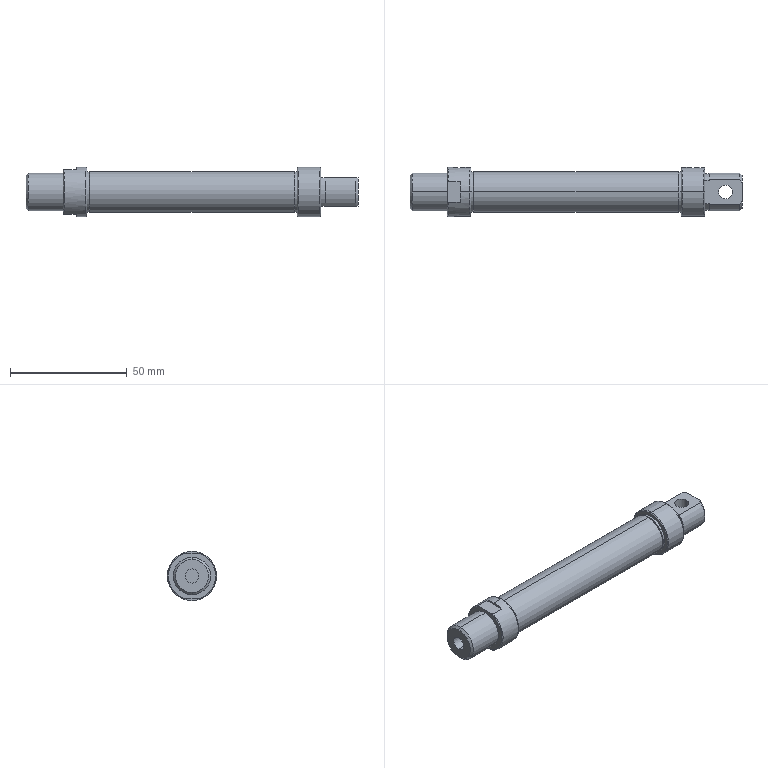Part | STEP file | 16MALB50_Body | 1 solid | 66 faces | box 142 x 21 x 21 mm | volume 18560 mm3 | cylinder 26 | plane 20 | cone 12 | torus 8 | commonest cylinder face diameters 16 x6 17.4 x6 4.134 x4 6 x4 21 x4 15.7 x2